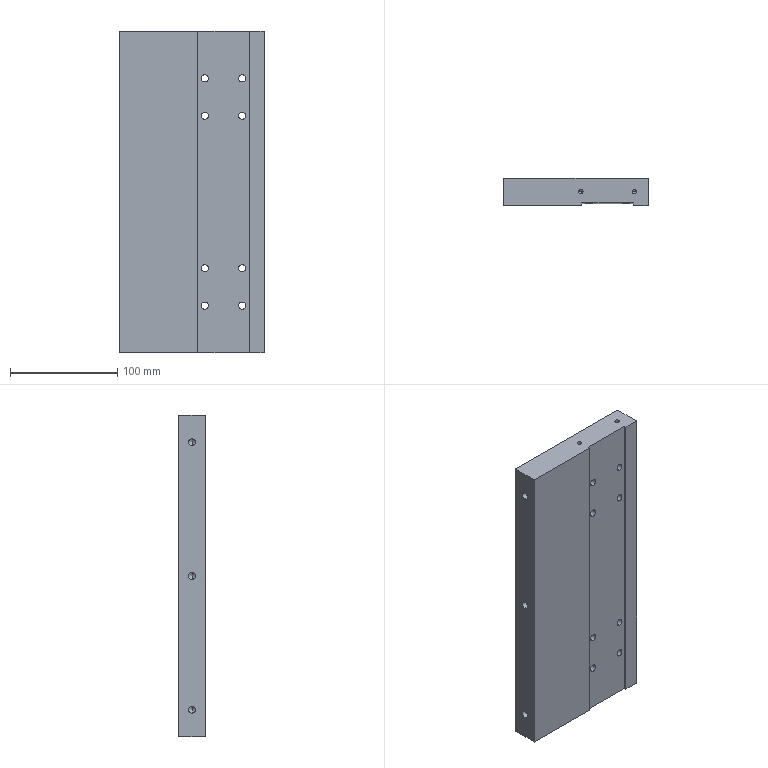Part | SolidWorks | features HoleWzd 3, Cut 1, Extrusion 1, MirrorPattern 1 | 1 solid | 82 faces | box 135 x 25 x 300 mm | volume 964423 mm3 | cylinder 48 | plane 18 | cone 16 | commonest cylinder face diameters 6.6 x16 11 x16 6.8 x12 4.2 x4